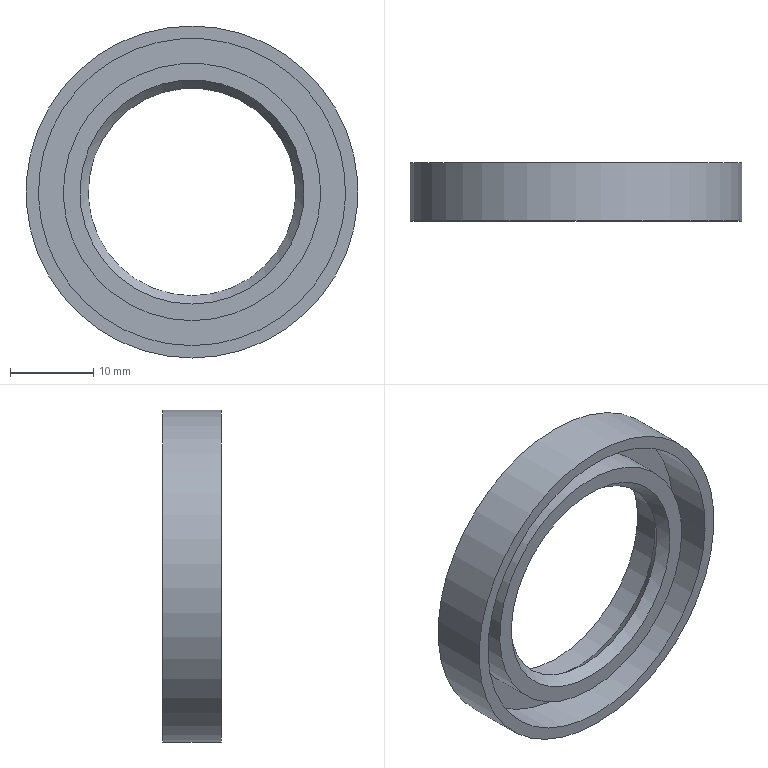Part | NX | features DATUM_CSYS 2, SKETCH 1, SWP104 1 | 1 solid | 11 faces | box 40 x 7 x 40 mm | volume 2796 mm3 | plane 5 | cylinder 4 | cone 2 | commonest cylinder face diameters 28 x1 31 x1 37 x1 40 x1
STEP:
#1=CARTESIAN_POINT('',(0.,0.,-18.5));
#2=VERTEX_POINT('',#1);
#3=CARTESIAN_POINT('',(0.,0.,0.));
#4=DIRECTION('',(0.,-1.,0.));
#5=DIRECTION('',(0.,0.,-1.));
#6=AXIS2_PLACEMENT_3D('',#3,#4,#5);
#7=CIRCLE('',#6,18.5);
#8=EDGE_CURVE('',#2,#2,#7,.T.);
#9=ORIENTED_EDGE('',*,*,#8,.F.);
#10=EDGE_LOOP('',(#9));
#11=FACE_BOUND('',#10,.T.);
#12=CARTESIAN_POINT('',(0.,0.,-20.));
#13=VERTEX_POINT('',#12);
#14=CARTESIAN_POINT('',(0.,0.,0.));
#15=DIRECTION('',(0.,-1.,0.));
#16=DIRECTION('',(0.,0.,-1.));
#17=AXIS2_PLACEMENT_3D('',#14,#15,#16);
#18=CIRCLE('',#17,20.);
#19=EDGE_CURVE('',#13,#13,#18,.T.);
#20=ORIENTED_EDGE('',*,*,#19,.T.);
#21=EDGE_LOOP('',(#20));
#22=FACE_BOUND('',#21,.T.);
#23=CARTESIAN_POINT('',(0.,0.,20.));
#24=DIRECTION('',(0.,1.,0.));
#25=DIRECTION('',(0.,0.,1.));
#26=AXIS2_PLACEMENT_3D('',#23,#24,#25);
#27=PLANE('',#26);
#28=ADVANCED_FACE('',(#11,#22),#27,.F.);
#29=CARTESIAN_POINT('',(0.,5.5,-18.5));
#30=VERTEX_POINT('',#29);
#31=CARTESIAN_POINT('',(0.,5.5,0.));
#32=DIRECTION('',(0.,-1.,0.));
#33=DIRECTION('',(0.,0.,-1.));
#34=AXIS2_PLACEMENT_3D('',#31,#32,#33);
#35=CIRCLE('',#34,18.5);
#36=EDGE_CURVE('',#30,#30,#35,.T.);
#37=ORIENTED_EDGE('',*,*,#36,.F.);
#38=EDGE_LOOP('',(#37));
#39=FACE_BOUND('',#38,.T.);
#40=ORIENTED_EDGE('',*,*,#8,.T.);
#41=EDGE_LOOP('',(#40));
#42=FACE_BOUND('',#41,.T.);
#43=CARTESIAN_POINT('',(0.,0.,0.));
#44=DIRECTION('',(0.,-1.,0.));
#45=DIRECTION('',(0.,0.,-1.));
#46=AXIS2_PLACEMENT_3D('',#43,#44,#45);
#47=CYLINDRICAL_SURFACE('',#46,18.5);
#48=ADVANCED_FACE('',(#39,#42),#47,.F.);
#49=CARTESIAN_POINT('',(0.,5.5,-15.5));
#50=VERTEX_POINT('',#49);
#51=CARTESIAN_POINT('',(0.,5.5,0.));
#52=DIRECTION('',(0.,-1.,0.));
#53=DIRECTION('',(0.,0.,-1.));
#54=AXIS2_PLACEMENT_3D('',#51,#52,#53);
#55=CIRCLE('',#54,15.5);
#56=EDGE_CURVE('',#50,#50,#55,.T.);
#57=ORIENTED_EDGE('',*,*,#56,.F.);
#58=EDGE_LOOP('',(#57));
#59=FACE_BOUND('',#58,.T.);
#60=ORIENTED_EDGE('',*,*,#36,.T.);
#61=EDGE_LOOP('',(#60));
#62=FACE_BOUND('',#61,.T.);
#63=CARTESIAN_POINT('',(0.,5.5,18.5));
#64=DIRECTION('',(0.,1.,0.));
#65=DIRECTION('',(0.,0.,1.));
#66=AXIS2_PLACEMENT_3D('',#63,#64,#65);
#67=PLANE('',#66);
#68=ADVANCED_FACE('',(#59,#62),#67,.F.);
#69=CARTESIAN_POINT('',(0.,1.,-15.5));
#70=VERTEX_POINT('',#69);
#71=CARTESIAN_POINT('',(0.,1.,0.));
#72=DIRECTION('',(0.,-1.,0.));
#73=DIRECTION('',(0.,0.,-1.));
#74=AXIS2_PLACEMENT_3D('',#71,#72,#73);
#75=CIRCLE('',#74,15.5);
#76=EDGE_CURVE('',#70,#70,#75,.T.);
#77=ORIENTED_EDGE('',*,*,#76,.F.);
#78=EDGE_LOOP('',(#77));
#79=FACE_BOUND('',#78,.T.);
#80=ORIENTED_EDGE('',*,*,#56,.T.);
#81=EDGE_LOOP('',(#80));
#82=FACE_BOUND('',#81,.T.);
#83=CARTESIAN_POINT('',(0.,0.,0.));
#84=DIRECTION('',(0.,-1.,0.));
#85=DIRECTION('',(0.,0.,-1.));
#86=AXIS2_PLACEMENT_3D('',#83,#84,#85);
#87=CYLINDRICAL_SURFACE('',#86,15.5);
#88=ADVANCED_FACE('',(#79,#82),#87,.T.);
#89=CARTESIAN_POINT('',(0.,1.,-13.5));
#90=VERTEX_POINT('',#89);
#91=CARTESIAN_POINT('',(0.,1.,0.));
#92=DIRECTION('',(0.,-1.,0.));
#93=DIRECTION('',(0.,0.,-1.));
#94=AXIS2_PLACEMENT_3D('',#91,#92,#93);
#95=CIRCLE('',#94,13.5);
#96=EDGE_CURVE('',#90,#90,#95,.T.);
#97=ORIENTED_EDGE('',*,*,#96,.F.);
#98=EDGE_LOOP('',(#97));
#99=FACE_BOUND('',#98,.T.);
#100=ORIENTED_EDGE('',*,*,#76,.T.);
#101=EDGE_LOOP('',(#100));
#102=FACE_BOUND('',#101,.T.);
#103=CARTESIAN_POINT('',(0.,1.,15.5));
#104=DIRECTION('',(0.,1.,0.));
#105=DIRECTION('',(0.,0.,1.));
#106=AXIS2_PLACEMENT_3D('',#103,#104,#105);
#107=PLANE('',#106);
#108=ADVANCED_FACE('',(#99,#102),#107,.F.);
#109=CARTESIAN_POINT('',(0.,2.25,-12.5));
#110=VERTEX_POINT('',#109);
#111=CARTESIAN_POINT('',(0.,2.25,0.));
#112=DIRECTION('',(0.,-1.,0.));
#113=DIRECTION('',(0.,0.,-1.));
#114=AXIS2_PLACEMENT_3D('',#111,#112,#113);
#115=CIRCLE('',#114,12.5);
#116=EDGE_CURVE('',#110,#110,#115,.T.);
#117=ORIENTED_EDGE('',*,*,#116,.F.);
#118=EDGE_LOOP('',(#117));
#119=FACE_BOUND('',#118,.T.);
#120=ORIENTED_EDGE('',*,*,#96,.T.);
#121=EDGE_LOOP('',(#120));
#122=FACE_BOUND('',#121,.T.);
#123=CARTESIAN_POINT('',(0.,1.,0.));
#124=DIRECTION('',(0.,-1.,0.));
#125=DIRECTION('',(0.,0.,-1.));
#126=AXIS2_PLACEMENT_3D('',#123,#124,#125);
#127=CONICAL_SURFACE('',#126,13.5,0.6747);
#128=ADVANCED_FACE('',(#119,#122),#127,.F.);
#129=CARTESIAN_POINT('',(0.,3.5,-13.5));
#130=VERTEX_POINT('',#129);
#131=CARTESIAN_POINT('',(0.,3.5,0.));
#132=DIRECTION('',(0.,-1.,0.));
#133=DIRECTION('',(0.,0.,-1.));
#134=AXIS2_PLACEMENT_3D('',#131,#132,#133);
#135=CIRCLE('',#134,13.5);
#136=EDGE_CURVE('',#130,#130,#135,.T.);
#137=ORIENTED_EDGE('',*,*,#136,.F.);
#138=EDGE_LOOP('',(#137));
#139=FACE_BOUND('',#138,.T.);
#140=ORIENTED_EDGE('',*,*,#116,.T.);
#141=EDGE_LOOP('',(#140));
#142=FACE_BOUND('',#141,.T.);
#143=CARTESIAN_POINT('',(0.,2.25,0.));
#144=DIRECTION('',(0.,1.,0.));
#145=DIRECTION('',(0.,0.,1.));
#146=AXIS2_PLACEMENT_3D('',#143,#144,#145);
#147=CONICAL_SURFACE('',#146,12.5,0.6747);
#148=ADVANCED_FACE('',(#139,#142),#147,.F.);
#149=CARTESIAN_POINT('',(0.,3.5,-14.));
#150=VERTEX_POINT('',#149);
#151=CARTESIAN_POINT('',(0.,3.5,0.));
#152=DIRECTION('',(0.,-1.,0.));
#153=DIRECTION('',(0.,0.,-1.));
#154=AXIS2_PLACEMENT_3D('',#151,#152,#153);
#155=CIRCLE('',#154,14.);
#156=EDGE_CURVE('',#150,#150,#155,.T.);
#157=ORIENTED_EDGE('',*,*,#156,.F.);
#158=EDGE_LOOP('',(#157));
#159=FACE_BOUND('',#158,.T.);
#160=ORIENTED_EDGE('',*,*,#136,.T.);
#161=EDGE_LOOP('',(#160));
#162=FACE_BOUND('',#161,.T.);
#163=CARTESIAN_POINT('',(0.,3.5,13.5));
#164=DIRECTION('',(0.,-1.,0.));
#165=DIRECTION('',(0.,0.,-1.));
#166=AXIS2_PLACEMENT_3D('',#163,#164,#165);
#167=PLANE('',#166);
#168=ADVANCED_FACE('',(#159,#162),#167,.F.);
#169=CARTESIAN_POINT('',(0.,7.,-14.));
#170=VERTEX_POINT('',#169);
#171=CARTESIAN_POINT('',(0.,7.,0.));
#172=DIRECTION('',(0.,-1.,0.));
#173=DIRECTION('',(0.,0.,-1.));
#174=AXIS2_PLACEMENT_3D('',#171,#172,#173);
#175=CIRCLE('',#174,14.);
#176=EDGE_CURVE('',#170,#170,#175,.T.);
#177=ORIENTED_EDGE('',*,*,#176,.F.);
#178=EDGE_LOOP('',(#177));
#179=FACE_BOUND('',#178,.T.);
#180=ORIENTED_EDGE('',*,*,#156,.T.);
#181=EDGE_LOOP('',(#180));
#182=FACE_BOUND('',#181,.T.);
#183=CARTESIAN_POINT('',(0.,0.,0.));
#184=DIRECTION('',(0.,-1.,0.));
#185=DIRECTION('',(0.,0.,-1.));
#186=AXIS2_PLACEMENT_3D('',#183,#184,#185);
#187=CYLINDRICAL_SURFACE('',#186,14.);
#188=ADVANCED_FACE('',(#179,#182),#187,.F.);
#189=CARTESIAN_POINT('',(0.,7.,-20.));
#190=VERTEX_POINT('',#189);
#191=CARTESIAN_POINT('',(0.,7.,0.));
#192=DIRECTION('',(0.,-1.,0.));
#193=DIRECTION('',(0.,0.,-1.));
#194=AXIS2_PLACEMENT_3D('',#191,#192,#193);
#195=CIRCLE('',#194,20.);
#196=EDGE_CURVE('',#190,#190,#195,.T.);
#197=ORIENTED_EDGE('',*,*,#196,.F.);
#198=EDGE_LOOP('',(#197));
#199=FACE_BOUND('',#198,.T.);
#200=ORIENTED_EDGE('',*,*,#176,.T.);
#201=EDGE_LOOP('',(#200));
#202=FACE_BOUND('',#201,.T.);
#203=CARTESIAN_POINT('',(0.,7.,14.));
#204=DIRECTION('',(0.,-1.,0.));
#205=DIRECTION('',(0.,0.,-1.));
#206=AXIS2_PLACEMENT_3D('',#203,#204,#205);
#207=PLANE('',#206);
#208=ADVANCED_FACE('',(#199,#202),#207,.F.);
#209=ORIENTED_EDGE('',*,*,#19,.F.);
#210=EDGE_LOOP('',(#209));
#211=FACE_BOUND('',#210,.T.);
#212=ORIENTED_EDGE('',*,*,#196,.T.);
#213=EDGE_LOOP('',(#212));
#214=FACE_BOUND('',#213,.T.);
#215=CARTESIAN_POINT('',(0.,0.,0.));
#216=DIRECTION('',(0.,-1.,0.));
#217=DIRECTION('',(0.,0.,-1.));
#218=AXIS2_PLACEMENT_3D('',#215,#216,#217);
#219=CYLINDRICAL_SURFACE('',#218,20.);
#220=ADVANCED_FACE('',(#211,#214),#219,.T.);
#221=CLOSED_SHELL('',(#28,#48,#68,#88,#108,#128,#148,#168,#188,#208,#220));
#222=MANIFOLD_SOLID_BREP('',#221);
#223=(LENGTH_UNIT()NAMED_UNIT(*)SI_UNIT(.MILLI.,.METRE.));
#224=UNCERTAINTY_MEASURE_WITH_UNIT(LENGTH_MEASURE(0.00001),#223,'','');
#225=(NAMED_UNIT(*)PLANE_ANGLE_UNIT()SI_UNIT($,.RADIAN.));
#226=(NAMED_UNIT(*)SI_UNIT($,.STERADIAN.)SOLID_ANGLE_UNIT());
#227=(GEOMETRIC_REPRESENTATION_CONTEXT(3)GLOBAL_UNCERTAINTY_ASSIGNED_CONTEXT((#224))GLOBAL_UNIT_ASSIGNED_CONTEXT((#223,#225,#226))REPRESENTATION_CONTEXT('',''));
#228=ADVANCED_BREP_SHAPE_REPRESENTATION('',(#222),#227);